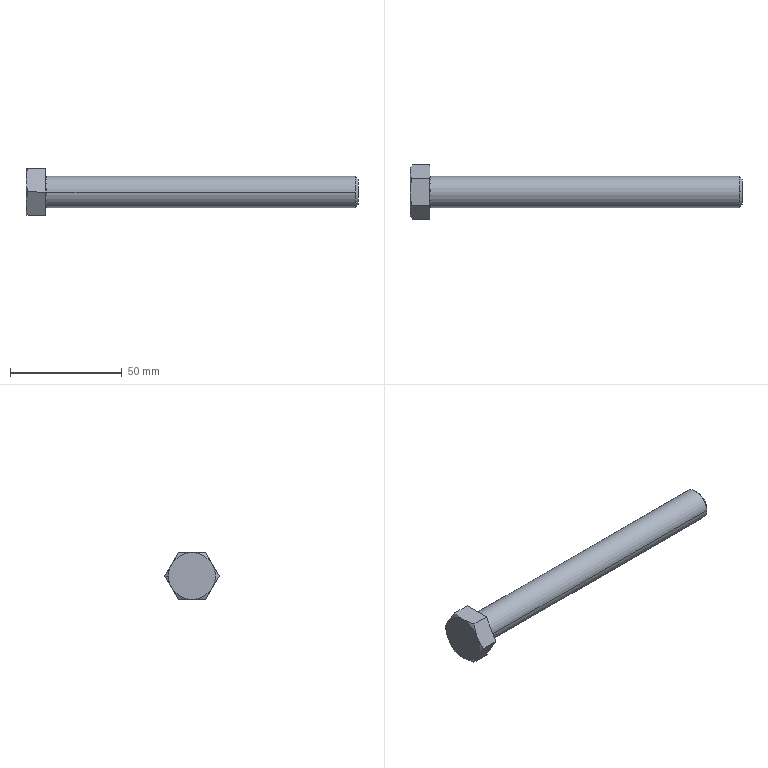Part | SolidWorks | features BaseBody 1 | 1 solid | 22 faces | box 148.8 x 24.249 x 21 mm | volume 24876 mm3 | cone 9 | plane 9 | spline 2 | cylinder 2 | commonest cylinder face diameters 14 x2
STEP:
#1=CARTESIAN_POINT('',(0.,0.,7.6));
#2=VERTEX_POINT('',#1);
#3=CARTESIAN_POINT('',(0.,0.,-7.6));
#4=VERTEX_POINT('',#3);
#5=CARTESIAN_POINT('',(0.,0.,7.6));
#6=CARTESIAN_POINT('',(0.,0.2323,7.6));
#7=CARTESIAN_POINT('',(0.,0.5793,7.584));
#8=CARTESIAN_POINT('',(0.,0.9819,7.538));
#9=CARTESIAN_POINT('',(0.,1.183,7.508));
#10=CARTESIAN_POINT('',(0.,1.268,7.493));
#11=CARTESIAN_POINT('',(0.,1.326,7.484));
#12=CARTESIAN_POINT('',(0.,1.353,7.479));
#13=CARTESIAN_POINT('',(0.,1.625,7.428));
#14=CARTESIAN_POINT('',(0.,1.984,7.344));
#15=CARTESIAN_POINT('',(0.,2.393,7.215));
#16=CARTESIAN_POINT('',(0.,2.596,7.143));
#17=CARTESIAN_POINT('',(0.,2.683,7.111));
#18=CARTESIAN_POINT('',(0.,2.74,7.089));
#19=CARTESIAN_POINT('',(0.,2.768,7.078));
#20=CARTESIAN_POINT('',(0.,3.036,6.972));
#21=CARTESIAN_POINT('',(0.,3.385,6.813));
#22=CARTESIAN_POINT('',(0.,3.777,6.597));
#23=CARTESIAN_POINT('',(0.,3.942,6.498));
#24=CARTESIAN_POINT('',(0.,4.051,6.431));
#25=CARTESIAN_POINT('',(0.,4.104,6.397));
#26=CARTESIAN_POINT('',(0.,4.598,6.074));
#27=CARTESIAN_POINT('',(0.,5.003,5.745));
#28=CARTESIAN_POINT('',(0.,5.559,5.189));
#29=CARTESIAN_POINT('',(0.,5.822,4.898));
#30=CARTESIAN_POINT('',(0.,6.101,4.536));
#31=CARTESIAN_POINT('',(0.,6.214,4.376));
#32=CARTESIAN_POINT('',(0.,6.289,4.268));
#33=CARTESIAN_POINT('',(0.,6.326,4.212));
#34=CARTESIAN_POINT('',(0.,6.502,3.944));
#35=CARTESIAN_POINT('',(0.,6.695,3.613));
#36=CARTESIAN_POINT('',(0.,6.891,3.21));
#37=CARTESIAN_POINT('',(0.,6.981,3.005));
#38=CARTESIAN_POINT('',(0.,7.018,2.917));
#39=CARTESIAN_POINT('',(0.,7.043,2.857));
#40=CARTESIAN_POINT('',(0.,7.055,2.826));
#41=CARTESIAN_POINT('',(0.,7.157,2.569));
#42=CARTESIAN_POINT('',(0.,7.276,2.22));
#43=CARTESIAN_POINT('',(0.,7.385,1.804));
#44=CARTESIAN_POINT('',(0.,7.431,1.594));
#45=CARTESIAN_POINT('',(0.,7.45,1.504));
#46=CARTESIAN_POINT('',(0.,7.462,1.443));
#47=CARTESIAN_POINT('',(0.,7.468,1.411));
#48=CARTESIAN_POINT('',(0.,7.558,0.9257));
#49=CARTESIAN_POINT('',(0.,7.6,0.4647));
#50=CARTESIAN_POINT('',(0.,7.6,-0.2323));
#51=CARTESIAN_POINT('',(0.,7.589,-0.464));
#52=CARTESIAN_POINT('',(0.,7.558,-0.8097));
#53=CARTESIAN_POINT('',(0.,7.538,-0.9822));
#54=CARTESIAN_POINT('',(0.,7.508,-1.183));
#55=CARTESIAN_POINT('',(0.,7.493,-1.269));
#56=CARTESIAN_POINT('',(0.,7.484,-1.326));
#57=CARTESIAN_POINT('',(0.,7.479,-1.353));
#58=CARTESIAN_POINT('',(0.,7.428,-1.625));
#59=CARTESIAN_POINT('',(0.,7.344,-1.984));
#60=CARTESIAN_POINT('',(0.,7.215,-2.393));
#61=CARTESIAN_POINT('',(0.,7.143,-2.596));
#62=CARTESIAN_POINT('',(0.,7.111,-2.683));
#63=CARTESIAN_POINT('',(0.,7.089,-2.74));
#64=CARTESIAN_POINT('',(0.,7.078,-2.768));
#65=CARTESIAN_POINT('',(0.,6.972,-3.036));
#66=CARTESIAN_POINT('',(0.,6.813,-3.385));
#67=CARTESIAN_POINT('',(0.,6.597,-3.777));
#68=CARTESIAN_POINT('',(0.,6.498,-3.942));
#69=CARTESIAN_POINT('',(0.,6.431,-4.051));
#70=CARTESIAN_POINT('',(0.,6.397,-4.104));
#71=CARTESIAN_POINT('',(0.,6.074,-4.598));
#72=CARTESIAN_POINT('',(0.,5.745,-5.003));
#73=CARTESIAN_POINT('',(0.,5.189,-5.559));
#74=CARTESIAN_POINT('',(0.,4.898,-5.822));
#75=CARTESIAN_POINT('',(0.,4.536,-6.101));
#76=CARTESIAN_POINT('',(0.,4.376,-6.214));
#77=CARTESIAN_POINT('',(0.,4.268,-6.289));
#78=CARTESIAN_POINT('',(0.,4.212,-6.326));
#79=CARTESIAN_POINT('',(0.,3.944,-6.502));
#80=CARTESIAN_POINT('',(0.,3.613,-6.695));
#81=CARTESIAN_POINT('',(0.,3.21,-6.891));
#82=CARTESIAN_POINT('',(0.,3.005,-6.981));
#83=CARTESIAN_POINT('',(0.,2.917,-7.018));
#84=CARTESIAN_POINT('',(0.,2.857,-7.043));
#85=CARTESIAN_POINT('',(0.,2.826,-7.055));
#86=CARTESIAN_POINT('',(0.,2.569,-7.157));
#87=CARTESIAN_POINT('',(0.,2.22,-7.276));
#88=CARTESIAN_POINT('',(0.,1.804,-7.385));
#89=CARTESIAN_POINT('',(0.,1.594,-7.431));
#90=CARTESIAN_POINT('',(0.,1.504,-7.45));
#91=CARTESIAN_POINT('',(0.,1.443,-7.462));
#92=CARTESIAN_POINT('',(0.,1.411,-7.468));
#93=CARTESIAN_POINT('',(0.,0.9262,-7.558));
#94=CARTESIAN_POINT('',(0.,0.4645,-7.6));
#95=CARTESIAN_POINT('',(0.,0.,-7.6));
#96=B_SPLINE_CURVE_WITH_KNOTS('',3,(#5,#6,#7,#8,#9,#10,#11,#12,#13,#14,#15,#16,#17,#18,#19,#20,#21,#22,#23,#24,#25,#26,#27,#28,#29,#30,#31,#32,#33,#34,#35,#36,#37,#38,#39,#40,#41,#42,#43,#44,#45,#46,#47,#48,#49,#50,#51,#52,#53,#54,#55,#56,#57,#58,#59,#60,#61,#62,#63,#64,#65,#66,#67,#68,#69,#70,#71,#72,#73,#74,#75,#76,#77,#78,#79,#80,#81,#82,#83,#84,#85,#86,#87,#88,#89,#90,#91,#92,#93,#94,#95),.UNSPECIFIED.,.F.,.F.,(4,1,1,1,2,2,1,1,1,2,2,1,1,2,2,2,1,1,2,2,1,1,1,2,2,1,1,1,2,2,2,2,1,1,2,2,1,1,1,2,2,1,1,2,2,2,1,1,2,2,1,1,1,2,2,1,1,1,2,2,4),(0.75,0.7656,0.7734,0.7773,0.7793,0.7812,0.7969,0.8047,0.8086,0.8105,0.8125,0.8281,0.8359,0.8398,0.8438,0.875,0.8906,0.8984,0.9023,0.9063,0.9219,0.9297,0.9336,0.9355,0.9375,0.9531,0.9609,0.9648,0.9668,0.9688,1.,1.016,1.023,1.027,1.029,1.031,1.047,1.055,1.059,1.061,1.063,1.078,1.086,1.09,1.094,1.125,1.141,1.148,1.152,1.156,1.172,1.18,1.184,1.186,1.188,1.203,1.211,1.215,1.217,1.219,1.25),.UNSPECIFIED.);
#97=EDGE_CURVE('',#2,#4,#96,.T.);
#98=ORIENTED_EDGE('',*,*,#97,.F.);
#99=CARTESIAN_POINT('',(0.6,0.,7.));
#100=VERTEX_POINT('',#99);
#101=CARTESIAN_POINT('',(0.6,0.,7.6));
#102=DIRECTION('',(0.,-1.,0.));
#103=DIRECTION('',(0.,0.,1.));
#104=AXIS2_PLACEMENT_3D('',#101,#102,#103);
#105=CIRCLE('',#104,0.6);
#106=EDGE_CURVE('',#2,#100,#105,.T.);
#107=ORIENTED_EDGE('',*,*,#106,.T.);
#108=CARTESIAN_POINT('',(0.6,7.,0.));
#109=VERTEX_POINT('',#108);
#110=CARTESIAN_POINT('',(0.6,0.,0.));
#111=DIRECTION('',(1.,0.,0.));
#112=DIRECTION('',(0.,1.,0.));
#113=AXIS2_PLACEMENT_3D('',#110,#111,#112);
#114=CIRCLE('',#113,7.);
#115=EDGE_CURVE('',#109,#100,#114,.T.);
#116=ORIENTED_EDGE('',*,*,#115,.F.);
#117=CARTESIAN_POINT('',(0.6,0.,-7.));
#118=VERTEX_POINT('',#117);
#119=CARTESIAN_POINT('',(0.6,0.,0.));
#120=DIRECTION('',(1.,0.,0.));
#121=DIRECTION('',(0.,1.,0.));
#122=AXIS2_PLACEMENT_3D('',#119,#120,#121);
#123=CIRCLE('',#122,7.);
#124=EDGE_CURVE('',#118,#109,#123,.T.);
#125=ORIENTED_EDGE('',*,*,#124,.F.);
#126=CARTESIAN_POINT('',(0.6,0.,-7.6));
#127=DIRECTION('',(0.,1.,0.));
#128=DIRECTION('',(0.,0.,-1.));
#129=AXIS2_PLACEMENT_3D('',#126,#127,#128);
#130=CIRCLE('',#129,0.6);
#131=EDGE_CURVE('',#4,#118,#130,.T.);
#132=ORIENTED_EDGE('',*,*,#131,.F.);
#133=EDGE_LOOP('',(#98,#107,#116,#125,#132));
#134=FACE_OUTER_BOUND('',#133,.T.);
#135=CARTESIAN_POINT('',(0.,0.,-7.6));
#136=CARTESIAN_POINT('',(0.,15.2,-7.6));
#137=CARTESIAN_POINT('',(0.,15.2,7.6));
#138=CARTESIAN_POINT('',(0.,0.,7.6));
#139=CARTESIAN_POINT('',(0.,0.,-7.249));
#140=CARTESIAN_POINT('',(0.,14.497,-7.249));
#141=CARTESIAN_POINT('',(0.,14.497,7.249));
#142=CARTESIAN_POINT('',(0.,0.,7.249));
#143=CARTESIAN_POINT('',(0.2485,0.,-7.));
#144=CARTESIAN_POINT('',(0.2485,14.,-7.));
#145=CARTESIAN_POINT('',(0.2485,14.,7.));
#146=CARTESIAN_POINT('',(0.2485,0.,7.));
#147=CARTESIAN_POINT('',(0.6,0.,-7.));
#148=CARTESIAN_POINT('',(0.6,14.,-7.));
#149=CARTESIAN_POINT('',(0.6,14.,7.));
#150=CARTESIAN_POINT('',(0.6,0.,7.));
#151=(BOUNDED_SURFACE()B_SPLINE_SURFACE(3,3,((#135,#136,#137,#138),(#139,#140,#141,#142),(#143,#144,#145,#146),(#147,#148,#149,#150)),.UNSPECIFIED.,.F.,.F.,.F.)B_SPLINE_SURFACE_WITH_KNOTS((4,4),(4,4),(0.,1.),(0.,1.),.UNSPECIFIED.)GEOMETRIC_REPRESENTATION_ITEM()RATIONAL_B_SPLINE_SURFACE(((1.,0.3333,0.3333,1.),(0.8047,0.2682,0.2682,0.8047),(0.8047,0.2682,0.2682,0.8047),(1.,0.3333,0.3333,1.)))REPRESENTATION_ITEM('')SURFACE());
#152=ADVANCED_FACE('',(#134),#151,.F.);
#153=ORIENTED_EDGE('',*,*,#115,.T.);
#154=CARTESIAN_POINT('',(0.6,-7.,0.));
#155=VERTEX_POINT('',#154);
#156=CARTESIAN_POINT('',(0.6,0.,0.));
#157=DIRECTION('',(1.,0.,0.));
#158=DIRECTION('',(0.,1.,0.));
#159=AXIS2_PLACEMENT_3D('',#156,#157,#158);
#160=CIRCLE('',#159,7.);
#161=EDGE_CURVE('',#100,#155,#160,.T.);
#162=ORIENTED_EDGE('',*,*,#161,.T.);
#163=CARTESIAN_POINT('',(138.773,-7.,0.));
#164=VERTEX_POINT('',#163);
#165=CARTESIAN_POINT('',(70.,-7.,0.));
#166=DIRECTION('',(1.,0.,0.));
#167=VECTOR('',#166,1000.);
#168=LINE('',#165,#167);
#169=EDGE_CURVE('',#155,#164,#168,.T.);
#170=ORIENTED_EDGE('',*,*,#169,.T.);
#171=CARTESIAN_POINT('',(138.773,0.,7.));
#172=VERTEX_POINT('',#171);
#173=CARTESIAN_POINT('',(138.773,0.,0.));
#174=DIRECTION('',(-1.,0.,0.));
#175=DIRECTION('',(0.,1.,0.));
#176=AXIS2_PLACEMENT_3D('',#173,#174,#175);
#177=CIRCLE('',#176,7.);
#178=EDGE_CURVE('',#164,#172,#177,.T.);
#179=ORIENTED_EDGE('',*,*,#178,.T.);
#180=CARTESIAN_POINT('',(138.773,7.,0.));
#181=VERTEX_POINT('',#180);
#182=CARTESIAN_POINT('',(138.773,0.,0.));
#183=DIRECTION('',(-1.,0.,0.));
#184=DIRECTION('',(0.,1.,0.));
#185=AXIS2_PLACEMENT_3D('',#182,#183,#184);
#186=CIRCLE('',#185,7.);
#187=EDGE_CURVE('',#172,#181,#186,.T.);
#188=ORIENTED_EDGE('',*,*,#187,.T.);
#189=CARTESIAN_POINT('',(70.,7.,0.));
#190=DIRECTION('',(1.,0.,0.));
#191=VECTOR('',#190,1000.);
#192=LINE('',#189,#191);
#193=EDGE_CURVE('',#109,#181,#192,.T.);
#194=ORIENTED_EDGE('',*,*,#193,.F.);
#195=EDGE_LOOP('',(#153,#162,#170,#179,#188,#194));
#196=FACE_OUTER_BOUND('',#195,.T.);
#197=CARTESIAN_POINT('',(70.,0.,0.));
#198=DIRECTION('',(1.,0.,0.));
#199=DIRECTION('',(0.,1.,0.));
#200=AXIS2_PLACEMENT_3D('',#197,#198,#199);
#201=CYLINDRICAL_SURFACE('',#200,7.);
#202=ADVANCED_FACE('',(#196),#201,.T.);
#203=CARTESIAN_POINT('',(140.,0.,5.773));
#204=VERTEX_POINT('',#203);
#205=CARTESIAN_POINT('',(140.,0.,-5.773));
#206=VERTEX_POINT('',#205);
#207=CARTESIAN_POINT('',(140.,0.,0.));
#208=DIRECTION('',(-1.,0.,0.));
#209=DIRECTION('',(0.,0.,1.));
#210=AXIS2_PLACEMENT_3D('',#207,#208,#209);
#211=CIRCLE('',#210,5.773);
#212=EDGE_CURVE('',#204,#206,#211,.T.);
#213=ORIENTED_EDGE('',*,*,#212,.T.);
#214=CARTESIAN_POINT('',(138.773,0.,-7.));
#215=VERTEX_POINT('',#214);
#216=CARTESIAN_POINT('',(138.773,0.,-7.));
#217=DIRECTION('',(-0.7071,0.,-0.7071));
#218=VECTOR('',#217,1000.);
#219=LINE('',#216,#218);
#220=EDGE_CURVE('',#206,#215,#219,.T.);
#221=ORIENTED_EDGE('',*,*,#220,.T.);
#222=CARTESIAN_POINT('',(138.773,0.,0.));
#223=DIRECTION('',(-1.,0.,0.));
#224=DIRECTION('',(0.,1.,0.));
#225=AXIS2_PLACEMENT_3D('',#222,#223,#224);
#226=CIRCLE('',#225,7.);
#227=EDGE_CURVE('',#181,#215,#226,.T.);
#228=ORIENTED_EDGE('',*,*,#227,.F.);
#229=ORIENTED_EDGE('',*,*,#187,.F.);
#230=CARTESIAN_POINT('',(138.773,0.,7.));
#231=DIRECTION('',(-0.7071,0.,0.7071));
#232=VECTOR('',#231,1000.);
#233=LINE('',#230,#232);
#234=EDGE_CURVE('',#204,#172,#233,.T.);
#235=ORIENTED_EDGE('',*,*,#234,.F.);
#236=EDGE_LOOP('',(#213,#221,#228,#229,#235));
#237=FACE_OUTER_BOUND('',#236,.T.);
#238=CARTESIAN_POINT('',(138.773,0.,0.));
#239=DIRECTION('',(-1.,0.,0.));
#240=DIRECTION('',(0.,0.,1.));
#241=AXIS2_PLACEMENT_3D('',#238,#239,#240);
#242=CONICAL_SURFACE('',#241,7.,0.7854);
#243=ADVANCED_FACE('',(#237),#242,.T.);
#244=CARTESIAN_POINT('',(-8.8,9.093,-5.25));
#245=VERTEX_POINT('',#244);
#246=CARTESIAN_POINT('',(-8.8,10.5,0.));
#247=VERTEX_POINT('',#246);
#248=CARTESIAN_POINT('',(-8.8,0.,0.));
#249=DIRECTION('',(1.,0.,0.));
#250=DIRECTION('',(0.,1.,0.));
#251=AXIS2_PLACEMENT_3D('',#248,#249,#250);
#252=CIRCLE('',#251,10.5);
#253=EDGE_CURVE('',#245,#247,#252,.T.);
#254=ORIENTED_EDGE('',*,*,#253,.T.);
#255=CARTESIAN_POINT('',(-7.862,12.124,0.));
#256=VERTEX_POINT('',#255);
#257=CARTESIAN_POINT('',(-7.857,12.134,0.));
#258=DIRECTION('',(0.5,0.866,0.));
#259=VECTOR('',#258,1000.);
#260=LINE('',#257,#259);
#261=EDGE_CURVE('',#247,#256,#260,.T.);
#262=ORIENTED_EDGE('',*,*,#261,.T.);
#263=CARTESIAN_POINT('',(-8.8,9.093,-5.25));
#264=CARTESIAN_POINT('',(-8.8,9.611,-4.354));
#265=CARTESIAN_POINT('',(-8.71,10.121,-3.47));
#266=CARTESIAN_POINT('',(-8.384,11.13,-1.722));
#267=CARTESIAN_POINT('',(-8.148,11.629,-0.8576));
#268=CARTESIAN_POINT('',(-7.862,12.124,0.));
#269=B_SPLINE_CURVE_WITH_KNOTS('',3,(#263,#264,#265,#266,#267,#268),.UNSPECIFIED.,.F.,.F.,(4,2,4),(0.,0.003067,0.006134),.UNSPECIFIED.);
#270=EDGE_CURVE('',#245,#256,#269,.T.);
#271=ORIENTED_EDGE('',*,*,#270,.F.);
#272=EDGE_LOOP('',(#254,#262,#271));
#273=FACE_OUTER_BOUND('',#272,.T.);
#274=CARTESIAN_POINT('',(-7.857,0.,0.));
#275=DIRECTION('',(1.,0.,0.));
#276=DIRECTION('',(0.,1.,0.));
#277=AXIS2_PLACEMENT_3D('',#274,#275,#276);
#278=CONICAL_SURFACE('',#277,12.134,1.047);
#279=ADVANCED_FACE('',(#273),#278,.T.);
#280=ORIENTED_EDGE('',*,*,#169,.F.);
#281=CARTESIAN_POINT('',(0.6,0.,0.));
#282=DIRECTION('',(1.,0.,0.));
#283=DIRECTION('',(0.,1.,0.));
#284=AXIS2_PLACEMENT_3D('',#281,#282,#283);
#285=CIRCLE('',#284,7.);
#286=EDGE_CURVE('',#155,#118,#285,.T.);
#287=ORIENTED_EDGE('',*,*,#286,.T.);
#288=ORIENTED_EDGE('',*,*,#124,.T.);
#289=ORIENTED_EDGE('',*,*,#193,.T.);
#290=ORIENTED_EDGE('',*,*,#227,.T.);
#291=CARTESIAN_POINT('',(138.773,0.,0.));
#292=DIRECTION('',(-1.,0.,0.));
#293=DIRECTION('',(0.,1.,0.));
#294=AXIS2_PLACEMENT_3D('',#291,#292,#293);
#295=CIRCLE('',#294,7.);
#296=EDGE_CURVE('',#215,#164,#295,.T.);
#297=ORIENTED_EDGE('',*,*,#296,.T.);
#298=EDGE_LOOP('',(#280,#287,#288,#289,#290,#297));
#299=FACE_OUTER_BOUND('',#298,.T.);
#300=CARTESIAN_POINT('',(70.,0.,0.));
#301=DIRECTION('',(1.,0.,0.));
#302=DIRECTION('',(0.,1.,0.));
#303=AXIS2_PLACEMENT_3D('',#300,#301,#302);
#304=CYLINDRICAL_SURFACE('',#303,7.);
#305=ADVANCED_FACE('',(#299),#304,.T.);
#306=ORIENTED_EDGE('',*,*,#106,.F.);
#307=CARTESIAN_POINT('',(0.,0.,-7.6));
#308=CARTESIAN_POINT('',(0.,-0.2323,-7.6));
#309=CARTESIAN_POINT('',(0.,-0.5793,-7.584));
#310=CARTESIAN_POINT('',(0.,-0.9819,-7.538));
#311=CARTESIAN_POINT('',(0.,-1.183,-7.508));
#312=CARTESIAN_POINT('',(0.,-1.268,-7.493));
#313=CARTESIAN_POINT('',(0.,-1.326,-7.484));
#314=CARTESIAN_POINT('',(0.,-1.353,-7.479));
#315=CARTESIAN_POINT('',(0.,-1.625,-7.428));
#316=CARTESIAN_POINT('',(0.,-1.984,-7.344));
#317=CARTESIAN_POINT('',(0.,-2.393,-7.215));
#318=CARTESIAN_POINT('',(0.,-2.596,-7.143));
#319=CARTESIAN_POINT('',(0.,-2.683,-7.111));
#320=CARTESIAN_POINT('',(0.,-2.74,-7.089));
#321=CARTESIAN_POINT('',(0.,-2.768,-7.078));
#322=CARTESIAN_POINT('',(0.,-3.036,-6.972));
#323=CARTESIAN_POINT('',(0.,-3.385,-6.813));
#324=CARTESIAN_POINT('',(0.,-3.777,-6.597));
#325=CARTESIAN_POINT('',(0.,-3.942,-6.498));
#326=CARTESIAN_POINT('',(0.,-4.051,-6.431));
#327=CARTESIAN_POINT('',(0.,-4.104,-6.397));
#328=CARTESIAN_POINT('',(0.,-4.598,-6.074));
#329=CARTESIAN_POINT('',(0.,-5.003,-5.745));
#330=CARTESIAN_POINT('',(0.,-5.559,-5.189));
#331=CARTESIAN_POINT('',(0.,-5.822,-4.898));
#332=CARTESIAN_POINT('',(0.,-6.101,-4.536));
#333=CARTESIAN_POINT('',(0.,-6.214,-4.376));
#334=CARTESIAN_POINT('',(0.,-6.289,-4.268));
#335=CARTESIAN_POINT('',(0.,-6.326,-4.212));
#336=CARTESIAN_POINT('',(0.,-6.502,-3.944));
#337=CARTESIAN_POINT('',(0.,-6.695,-3.613));
#338=CARTESIAN_POINT('',(0.,-6.891,-3.21));
#339=CARTESIAN_POINT('',(0.,-6.981,-3.005));
#340=CARTESIAN_POINT('',(0.,-7.018,-2.917));
#341=CARTESIAN_POINT('',(0.,-7.043,-2.857));
#342=CARTESIAN_POINT('',(0.,-7.055,-2.826));
#343=CARTESIAN_POINT('',(0.,-7.157,-2.569));
#344=CARTESIAN_POINT('',(0.,-7.276,-2.22));
#345=CARTESIAN_POINT('',(0.,-7.385,-1.804));
#346=CARTESIAN_POINT('',(0.,-7.431,-1.594));
#347=CARTESIAN_POINT('',(0.,-7.45,-1.504));
#348=CARTESIAN_POINT('',(0.,-7.462,-1.443));
#349=CARTESIAN_POINT('',(0.,-7.468,-1.411));
#350=CARTESIAN_POINT('',(0.,-7.558,-0.9262));
#351=CARTESIAN_POINT('',(0.,-7.6,-0.4645));
#352=CARTESIAN_POINT('',(0.,-7.6,0.2323));
#353=CARTESIAN_POINT('',(0.,-7.584,0.5793));
#354=CARTESIAN_POINT('',(0.,-7.538,0.9819));
#355=CARTESIAN_POINT('',(0.,-7.508,1.183));
#356=CARTESIAN_POINT('',(0.,-7.493,1.268));
#357=CARTESIAN_POINT('',(0.,-7.484,1.326));
#358=CARTESIAN_POINT('',(0.,-7.479,1.353));
#359=CARTESIAN_POINT('',(0.,-7.428,1.625));
#360=CARTESIAN_POINT('',(0.,-7.344,1.984));
#361=CARTESIAN_POINT('',(0.,-7.215,2.393));
#362=CARTESIAN_POINT('',(0.,-7.143,2.596));
#363=CARTESIAN_POINT('',(0.,-7.111,2.683));
#364=CARTESIAN_POINT('',(0.,-7.089,2.74));
#365=CARTESIAN_POINT('',(0.,-7.078,2.768));
#366=CARTESIAN_POINT('',(0.,-6.972,3.036));
#367=CARTESIAN_POINT('',(0.,-6.813,3.385));
#368=CARTESIAN_POINT('',(0.,-6.597,3.777));
#369=CARTESIAN_POINT('',(0.,-6.498,3.942));
#370=CARTESIAN_POINT('',(0.,-6.431,4.051));
#371=CARTESIAN_POINT('',(0.,-6.397,4.104));
#372=CARTESIAN_POINT('',(0.,-6.074,4.598));
#373=CARTESIAN_POINT('',(0.,-5.745,5.003));
#374=CARTESIAN_POINT('',(0.,-5.189,5.559));
#375=CARTESIAN_POINT('',(0.,-4.898,5.822));
#376=CARTESIAN_POINT('',(0.,-4.536,6.101));
#377=CARTESIAN_POINT('',(0.,-4.376,6.214));
#378=CARTESIAN_POINT('',(0.,-4.268,6.289));
#379=CARTESIAN_POINT('',(0.,-4.212,6.326));
#380=CARTESIAN_POINT('',(0.,-3.944,6.502));
#381=CARTESIAN_POINT('',(0.,-3.613,6.695));
#382=CARTESIAN_POINT('',(0.,-3.21,6.891));
#383=CARTESIAN_POINT('',(0.,-3.005,6.981));
#384=CARTESIAN_POINT('',(0.,-2.917,7.018));
#385=CARTESIAN_POINT('',(0.,-2.857,7.043));
#386=CARTESIAN_POINT('',(0.,-2.826,7.055));
#387=CARTESIAN_POINT('',(0.,-2.569,7.157));
#388=CARTESIAN_POINT('',(0.,-2.22,7.276));
#389=CARTESIAN_POINT('',(0.,-1.804,7.385));
#390=CARTESIAN_POINT('',(0.,-1.594,7.431));
#391=CARTESIAN_POINT('',(0.,-1.504,7.45));
#392=CARTESIAN_POINT('',(0.,-1.443,7.462));
#393=CARTESIAN_POINT('',(0.,-1.411,7.468));
#394=CARTESIAN_POINT('',(0.,-0.9262,7.558));
#395=CARTESIAN_POINT('',(0.,-0.4645,7.6));
#396=CARTESIAN_POINT('',(0.,0.,7.6));
#397=B_SPLINE_CURVE_WITH_KNOTS('',3,(#307,#308,#309,#310,#311,#312,#313,#314,#315,#316,#317,#318,#319,#320,#321,#322,#323,#324,#325,#326,#327,#328,#329,#330,#331,#332,#333,#334,#335,#336,#337,#338,#339,#340,#341,#342,#343,#344,#345,#346,#347,#348,#349,#350,#351,#352,#353,#354,#355,#356,#357,#358,#359,#360,#361,#362,#363,#364,#365,#366,#367,#368,#369,#370,#371,#372,#373,#374,#375,#376,#377,#378,#379,#380,#381,#382,#383,#384,#385,#386,#387,#388,#389,#390,#391,#392,#393,#394,#395,#396),.UNSPECIFIED.,.F.,.F.,(4,1,1,1,2,2,1,1,1,2,2,1,1,2,2,2,1,1,2,2,1,1,1,2,2,1,1,1,2,2,2,1,1,1,2,2,1,1,1,2,2,1,1,2,2,2,1,1,2,2,1,1,1,2,2,1,1,1,2,2,4),(0.25,0.2656,0.2734,0.2773,0.2793,0.2812,0.2969,0.3047,0.3086,0.3105,0.3125,0.3281,0.3359,0.3398,0.3437,0.375,0.3906,0.3984,0.4023,0.4062,0.4219,0.4297,0.4336,0.4355,0.4375,0.4531,0.4609,0.4648,0.4668,0.4687,0.5,0.5156,0.5234,0.5273,0.5293,0.5312,0.5469,0.5547,0.5586,0.5605,0.5625,0.5781,0.5859,0.5898,0.5938,0.625,0.6406,0.6484,0.6523,0.6562,0.6719,0.6797,0.6836,0.6855,0.6875,0.7031,0.7109,0.7148,0.7168,0.7188,0.75),.UNSPECIFIED.);
#398=EDGE_CURVE('',#4,#2,#397,.T.);
#399=ORIENTED_EDGE('',*,*,#398,.F.);
#400=ORIENTED_EDGE('',*,*,#131,.T.);
#401=ORIENTED_EDGE('',*,*,#286,.F.);
#402=ORIENTED_EDGE('',*,*,#161,.F.);
#403=EDGE_LOOP('',(#306,#399,#400,#401,#402));
#404=FACE_OUTER_BOUND('',#403,.T.);
#405=CARTESIAN_POINT('',(0.,0.,7.6));
#406=CARTESIAN_POINT('',(0.,-15.2,7.6));
#407=CARTESIAN_POINT('',(0.,-15.2,-7.6));
#408=CARTESIAN_POINT('',(0.,0.,-7.6));
#409=CARTESIAN_POINT('',(0.,0.,7.249));
#410=CARTESIAN_POINT('',(0.,-14.497,7.249));
#411=CARTESIAN_POINT('',(0.,-14.497,-7.249));
#412=CARTESIAN_POINT('',(0.,0.,-7.249));
#413=CARTESIAN_POINT('',(0.2485,0.,7.));
#414=CARTESIAN_POINT('',(0.2485,-14.,7.));
#415=CARTESIAN_POINT('',(0.2485,-14.,-7.));
#416=CARTESIAN_POINT('',(0.2485,0.,-7.));
#417=CARTESIAN_POINT('',(0.6,0.,7.));
#418=CARTESIAN_POINT('',(0.6,-14.,7.));
#419=CARTESIAN_POINT('',(0.6,-14.,-7.));
#420=CARTESIAN_POINT('',(0.6,0.,-7.));
#421=(BOUNDED_SURFACE()B_SPLINE_SURFACE(3,3,((#405,#406,#407,#408),(#409,#410,#411,#412),(#413,#414,#415,#416),(#417,#418,#419,#420)),.UNSPECIFIED.,.F.,.F.,.F.)B_SPLINE_SURFACE_WITH_KNOTS((4,4),(4,4),(0.,1.),(0.,1.),.UNSPECIFIED.)GEOMETRIC_REPRESENTATION_ITEM()RATIONAL_B_SPLINE_SURFACE(((1.,0.3333,0.3333,1.),(0.8047,0.2682,0.2682,0.8047),(0.8047,0.2682,0.2682,0.8047),(1.,0.3333,0.3333,1.)))REPRESENTATION_ITEM('')SURFACE());
#422=ADVANCED_FACE('',(#404),#421,.F.);
#423=ORIENTED_EDGE('',*,*,#220,.F.);
#424=CARTESIAN_POINT('',(140.,0.,0.));
#425=DIRECTION('',(-1.,0.,0.));
#426=DIRECTION('',(0.,0.,1.));
#427=AXIS2_PLACEMENT_3D('',#424,#425,#426);
#428=CIRCLE('',#427,5.773);
#429=EDGE_CURVE('',#206,#204,#428,.T.);
#430=ORIENTED_EDGE('',*,*,#429,.T.);
#431=ORIENTED_EDGE('',*,*,#234,.T.);
#432=ORIENTED_EDGE('',*,*,#178,.F.);
#433=ORIENTED_EDGE('',*,*,#296,.F.);
#434=EDGE_LOOP('',(#423,#430,#431,#432,#433));
#435=FACE_OUTER_BOUND('',#434,.T.);
#436=CARTESIAN_POINT('',(138.773,0.,0.));
#437=DIRECTION('',(-1.,0.,0.));
#438=DIRECTION('',(0.,0.,1.));
#439=AXIS2_PLACEMENT_3D('',#436,#437,#438);
#440=CONICAL_SURFACE('',#439,7.,0.7854);
#441=ADVANCED_FACE('',(#435),#440,.T.);
#442=ORIENTED_EDGE('',*,*,#398,.T.);
#443=ORIENTED_EDGE('',*,*,#97,.T.);
#444=EDGE_LOOP('',(#442,#443));
#445=FACE_BOUND('',#444,.T.);
#446=CARTESIAN_POINT('',(0.,-6.062,-10.5));
#447=VERTEX_POINT('',#446);
#448=CARTESIAN_POINT('',(0.,6.062,-10.5));
#449=VERTEX_POINT('',#448);
#450=CARTESIAN_POINT('',(0.,0.,-10.5));
#451=DIRECTION('',(0.,1.,0.));
#452=VECTOR('',#451,1000.);
#453=LINE('',#450,#452);
#454=EDGE_CURVE('',#447,#449,#453,.T.);
#455=ORIENTED_EDGE('',*,*,#454,.T.);
#456=CARTESIAN_POINT('',(0.,12.124,0.));
#457=VERTEX_POINT('',#456);
#458=CARTESIAN_POINT('',(0.,6.062,-10.5));
#459=DIRECTION('',(0.,0.5,0.866));
#460=VECTOR('',#459,1000.);
#461=LINE('',#458,#460);
#462=EDGE_CURVE('',#449,#457,#461,.T.);
#463=ORIENTED_EDGE('',*,*,#462,.T.);
#464=CARTESIAN_POINT('',(0.,6.062,10.5));
#465=VERTEX_POINT('',#464);
#466=CARTESIAN_POINT('',(0.,12.124,0.));
#467=DIRECTION('',(0.,-0.5,0.866));
#468=VECTOR('',#467,1000.);
#469=LINE('',#466,#468);
#470=EDGE_CURVE('',#457,#465,#469,.T.);
#471=ORIENTED_EDGE('',*,*,#470,.T.);
#472=CARTESIAN_POINT('',(0.,-6.062,10.5));
#473=VERTEX_POINT('',#472);
#474=CARTESIAN_POINT('',(0.,0.,10.5));
#475=DIRECTION('',(0.,-1.,0.));
#476=VECTOR('',#475,1000.);
#477=LINE('',#474,#476);
#478=EDGE_CURVE('',#465,#473,#477,.T.);
#479=ORIENTED_EDGE('',*,*,#478,.T.);
#480=CARTESIAN_POINT('',(0.,-12.124,0.));
#481=VERTEX_POINT('',#480);
#482=CARTESIAN_POINT('',(0.,-6.062,10.5));
#483=DIRECTION('',(0.,-0.5,-0.866));
#484=VECTOR('',#483,1000.);
#485=LINE('',#482,#484);
#486=EDGE_CURVE('',#473,#481,#485,.T.);
#487=ORIENTED_EDGE('',*,*,#486,.T.);
#488=CARTESIAN_POINT('',(0.,-12.124,0.));
#489=DIRECTION('',(0.,0.5,-0.866));
#490=VECTOR('',#489,1000.);
#491=LINE('',#488,#490);
#492=EDGE_CURVE('',#481,#447,#491,.T.);
#493=ORIENTED_EDGE('',*,*,#492,.T.);
#494=EDGE_LOOP('',(#455,#463,#471,#479,#487,#493));
#495=FACE_OUTER_BOUND('',#494,.T.);
#496=CARTESIAN_POINT('',(0.,0.,0.));
#497=DIRECTION('',(1.,0.,0.));
#498=DIRECTION('',(0.,1.,0.));
#499=AXIS2_PLACEMENT_3D('',#496,#497,#498);
#500=PLANE('',#499);
#501=ADVANCED_FACE('',(#445,#495),#500,.T.);
#502=ORIENTED_EDGE('',*,*,#212,.F.);
#503=ORIENTED_EDGE('',*,*,#429,.F.);
#504=EDGE_LOOP('',(#502,#503));
#505=FACE_OUTER_BOUND('',#504,.T.);
#506=CARTESIAN_POINT('',(140.,3.5,0.));
#507=DIRECTION('',(1.,0.,0.));
#508=DIRECTION('',(0.,1.,0.));
#509=AXIS2_PLACEMENT_3D('',#506,#507,#508);
#510=PLANE('',#509);
#511=ADVANCED_FACE('',(#505),#510,.T.);
#512=CARTESIAN_POINT('',(-7.862,6.062,-10.5));
#513=VERTEX_POINT('',#512);
#514=CARTESIAN_POINT('',(0.,6.062,-10.5));
#515=DIRECTION('',(-1.,0.,0.));
#516=VECTOR('',#515,1000.);
#517=LINE('',#514,#516);
#518=EDGE_CURVE('',#449,#513,#517,.T.);
#519=ORIENTED_EDGE('',*,*,#518,.T.);
#520=CARTESIAN_POINT('',(-7.862,6.062,-10.5));
#521=CARTESIAN_POINT('',(-8.148,6.557,-9.642));
#522=CARTESIAN_POINT('',(-8.384,7.056,-8.778));
#523=CARTESIAN_POINT('',(-8.71,8.066,-7.03));
#524=CARTESIAN_POINT('',(-8.8,8.576,-6.146));
#525=CARTESIAN_POINT('',(-8.8,9.093,-5.25));
#526=B_SPLINE_CURVE_WITH_KNOTS('',3,(#520,#521,#522,#523,#524,#525),.UNSPECIFIED.,.F.,.F.,(4,2,4),(0.,0.003067,0.006134),.UNSPECIFIED.);
#527=EDGE_CURVE('',#513,#245,#526,.T.);
#528=ORIENTED_EDGE('',*,*,#527,.T.);
#529=ORIENTED_EDGE('',*,*,#270,.T.);
#530=CARTESIAN_POINT('',(0.,12.124,0.));
#531=DIRECTION('',(1.,0.,0.));
#532=VECTOR('',#531,1000.);
#533=LINE('',#530,#532);
#534=EDGE_CURVE('',#256,#457,#533,.T.);
#535=ORIENTED_EDGE('',*,*,#534,.T.);
#536=ORIENTED_EDGE('',*,*,#462,.F.);
#537=EDGE_LOOP('',(#519,#528,#529,#535,#536));
#538=FACE_OUTER_BOUND('',#537,.T.);
#539=CARTESIAN_POINT('',(0.,6.062,-10.5));
#540=DIRECTION('',(0.,0.866,-0.5));
#541=DIRECTION('',(0.,0.5,0.866));
#542=AXIS2_PLACEMENT_3D('',#539,#540,#541);
#543=PLANE('',#542);
#544=ADVANCED_FACE('',(#538),#543,.T.);
#545=ORIENTED_EDGE('',*,*,#454,.F.);
#546=CARTESIAN_POINT('',(-7.862,-6.062,-10.5));
#547=VERTEX_POINT('',#546);
#548=CARTESIAN_POINT('',(0.,-6.062,-10.5));
#549=DIRECTION('',(-1.,0.,0.));
#550=VECTOR('',#549,1000.);
#551=LINE('',#548,#550);
#552=EDGE_CURVE('',#447,#547,#551,.T.);
#553=ORIENTED_EDGE('',*,*,#552,.T.);
#554=CARTESIAN_POINT('',(-8.8,0.,-10.5));
#555=VERTEX_POINT('',#554);
#556=CARTESIAN_POINT('',(-7.862,-6.062,-10.5));
#557=CARTESIAN_POINT('',(-8.148,-5.072,-10.5));
#558=CARTESIAN_POINT('',(-8.384,-4.074,-10.5));
#559=CARTESIAN_POINT('',(-8.71,-2.055,-10.5));
#560=CARTESIAN_POINT('',(-8.8,-1.035,-10.5));
#561=CARTESIAN_POINT('',(-8.8,0.,-10.5));
#562=B_SPLINE_CURVE_WITH_KNOTS('',3,(#556,#557,#558,#559,#560,#561),.UNSPECIFIED.,.F.,.F.,(4,2,4),(0.,0.003067,0.006134),.UNSPECIFIED.);
#563=EDGE_CURVE('',#547,#555,#562,.T.);
#564=ORIENTED_EDGE('',*,*,#563,.T.);
#565=CARTESIAN_POINT('',(-8.8,0.,-10.5));
#566=CARTESIAN_POINT('',(-8.8,1.035,-10.5));
#567=CARTESIAN_POINT('',(-8.71,2.055,-10.5));
#568=CARTESIAN_POINT('',(-8.384,4.074,-10.5));
#569=CARTESIAN_POINT('',(-8.148,5.072,-10.5));
#570=CARTESIAN_POINT('',(-7.862,6.062,-10.5));
#571=B_SPLINE_CURVE_WITH_KNOTS('',3,(#565,#566,#567,#568,#569,#570),.UNSPECIFIED.,.F.,.F.,(4,2,4),(0.,0.003067,0.006134),.UNSPECIFIED.);
#572=EDGE_CURVE('',#555,#513,#571,.T.);
#573=ORIENTED_EDGE('',*,*,#572,.T.);
#574=ORIENTED_EDGE('',*,*,#518,.F.);
#575=EDGE_LOOP('',(#545,#553,#564,#573,#574));
#576=FACE_OUTER_BOUND('',#575,.T.);
#577=CARTESIAN_POINT('',(0.,-6.062,-10.5));
#578=DIRECTION('',(0.,0.,-1.));
#579=DIRECTION('',(0.,1.,0.));
#580=AXIS2_PLACEMENT_3D('',#577,#578,#579);
#581=PLANE('',#580);
#582=ADVANCED_FACE('',(#576),#581,.T.);
#583=ORIENTED_EDGE('',*,*,#492,.F.);
#584=CARTESIAN_POINT('',(-7.862,-12.124,0.));
#585=VERTEX_POINT('',#584);
#586=CARTESIAN_POINT('',(0.,-12.124,0.));
#587=DIRECTION('',(-1.,0.,0.));
#588=VECTOR('',#587,1000.);
#589=LINE('',#586,#588);
#590=EDGE_CURVE('',#481,#585,#589,.T.);
#591=ORIENTED_EDGE('',*,*,#590,.T.);
#592=CARTESIAN_POINT('',(-8.8,-9.093,-5.25));
#593=VERTEX_POINT('',#592);
#594=CARTESIAN_POINT('',(-7.862,-12.124,0.));
#595=CARTESIAN_POINT('',(-8.148,-11.629,-0.8576));
#596=CARTESIAN_POINT('',(-8.384,-11.13,-1.722));
#597=CARTESIAN_POINT('',(-8.71,-10.121,-3.47));
#598=CARTESIAN_POINT('',(-8.8,-9.611,-4.354));
#599=CARTESIAN_POINT('',(-8.8,-9.093,-5.25));
#600=B_SPLINE_CURVE_WITH_KNOTS('',3,(#594,#595,#596,#597,#598,#599),.UNSPECIFIED.,.F.,.F.,(4,2,4),(0.,0.003067,0.006134),.UNSPECIFIED.);
#601=EDGE_CURVE('',#585,#593,#600,.T.);
#602=ORIENTED_EDGE('',*,*,#601,.T.);
#603=CARTESIAN_POINT('',(-8.8,-9.093,-5.25));
#604=CARTESIAN_POINT('',(-8.8,-8.576,-6.146));
#605=CARTESIAN_POINT('',(-8.71,-8.066,-7.03));
#606=CARTESIAN_POINT('',(-8.384,-7.056,-8.778));
#607=CARTESIAN_POINT('',(-8.148,-6.557,-9.642));
#608=CARTESIAN_POINT('',(-7.862,-6.062,-10.5));
#609=B_SPLINE_CURVE_WITH_KNOTS('',3,(#603,#604,#605,#606,#607,#608),.UNSPECIFIED.,.F.,.F.,(4,2,4),(0.,0.003067,0.006134),.UNSPECIFIED.);
#610=EDGE_CURVE('',#593,#547,#609,.T.);
#611=ORIENTED_EDGE('',*,*,#610,.T.);
#612=ORIENTED_EDGE('',*,*,#552,.F.);
#613=EDGE_LOOP('',(#583,#591,#602,#611,#612));
#614=FACE_OUTER_BOUND('',#613,.T.);
#615=CARTESIAN_POINT('',(0.,-12.124,0.));
#616=DIRECTION('',(0.,-0.866,-0.5));
#617=DIRECTION('',(0.,0.5,-0.866));
#618=AXIS2_PLACEMENT_3D('',#615,#616,#617);
#619=PLANE('',#618);
#620=ADVANCED_FACE('',(#614),#619,.T.);
#621=ORIENTED_EDGE('',*,*,#486,.F.);
#622=CARTESIAN_POINT('',(-7.862,-6.062,10.5));
#623=VERTEX_POINT('',#622);
#624=CARTESIAN_POINT('',(0.,-6.062,10.5));
#625=DIRECTION('',(-1.,0.,0.));
#626=VECTOR('',#625,1000.);
#627=LINE('',#624,#626);
#628=EDGE_CURVE('',#473,#623,#627,.T.);
#629=ORIENTED_EDGE('',*,*,#628,.T.);
#630=CARTESIAN_POINT('',(-8.8,-9.093,5.25));
#631=VERTEX_POINT('',#630);
#632=CARTESIAN_POINT('',(-7.862,-6.062,10.5));
#633=CARTESIAN_POINT('',(-8.148,-6.557,9.642));
#634=CARTESIAN_POINT('',(-8.384,-7.056,8.778));
#635=CARTESIAN_POINT('',(-8.71,-8.066,7.03));
#636=CARTESIAN_POINT('',(-8.8,-8.576,6.146));
#637=CARTESIAN_POINT('',(-8.8,-9.093,5.25));
#638=B_SPLINE_CURVE_WITH_KNOTS('',3,(#632,#633,#634,#635,#636,#637),.UNSPECIFIED.,.F.,.F.,(4,2,4),(0.,0.003067,0.006134),.UNSPECIFIED.);
#639=EDGE_CURVE('',#623,#631,#638,.T.);
#640=ORIENTED_EDGE('',*,*,#639,.T.);
#641=CARTESIAN_POINT('',(-8.8,-9.093,5.25));
#642=CARTESIAN_POINT('',(-8.8,-9.611,4.354));
#643=CARTESIAN_POINT('',(-8.71,-10.121,3.47));
#644=CARTESIAN_POINT('',(-8.384,-11.13,1.722));
#645=CARTESIAN_POINT('',(-8.148,-11.629,0.8576));
#646=CARTESIAN_POINT('',(-7.862,-12.124,0.));
#647=B_SPLINE_CURVE_WITH_KNOTS('',3,(#641,#642,#643,#644,#645,#646),.UNSPECIFIED.,.F.,.F.,(4,2,4),(0.,0.003067,0.006134),.UNSPECIFIED.);
#648=EDGE_CURVE('',#631,#585,#647,.T.);
#649=ORIENTED_EDGE('',*,*,#648,.T.);
#650=ORIENTED_EDGE('',*,*,#590,.F.);
#651=EDGE_LOOP('',(#621,#629,#640,#649,#650));
#652=FACE_OUTER_BOUND('',#651,.T.);
#653=CARTESIAN_POINT('',(0.,-6.062,10.5));
#654=DIRECTION('',(0.,-0.866,0.5));
#655=DIRECTION('',(0.,-0.5,-0.866));
#656=AXIS2_PLACEMENT_3D('',#653,#654,#655);
#657=PLANE('',#656);
#658=ADVANCED_FACE('',(#652),#657,.T.);
#659=CARTESIAN_POINT('',(-7.862,6.062,10.5));
#660=VERTEX_POINT('',#659);
#661=CARTESIAN_POINT('',(0.,6.062,10.5));
#662=DIRECTION('',(-1.,0.,0.));
#663=VECTOR('',#662,1000.);
#664=LINE('',#661,#663);
#665=EDGE_CURVE('',#465,#660,#664,.T.);
#666=ORIENTED_EDGE('',*,*,#665,.T.);
#667=CARTESIAN_POINT('',(-8.8,0.,10.5));
#668=VERTEX_POINT('',#667);
#669=CARTESIAN_POINT('',(-7.862,6.062,10.5));
#670=CARTESIAN_POINT('',(-8.148,5.072,10.5));
#671=CARTESIAN_POINT('',(-8.384,4.074,10.5));
#672=CARTESIAN_POINT('',(-8.71,2.055,10.5));
#673=CARTESIAN_POINT('',(-8.8,1.035,10.5));
#674=CARTESIAN_POINT('',(-8.8,0.,10.5));
#675=B_SPLINE_CURVE_WITH_KNOTS('',3,(#669,#670,#671,#672,#673,#674),.UNSPECIFIED.,.F.,.F.,(4,2,4),(0.,0.003067,0.006134),.UNSPECIFIED.);
#676=EDGE_CURVE('',#660,#668,#675,.T.);
#677=ORIENTED_EDGE('',*,*,#676,.T.);
#678=CARTESIAN_POINT('',(-8.8,0.,10.5));
#679=CARTESIAN_POINT('',(-8.8,-1.035,10.5));
#680=CARTESIAN_POINT('',(-8.71,-2.055,10.5));
#681=CARTESIAN_POINT('',(-8.384,-4.074,10.5));
#682=CARTESIAN_POINT('',(-8.148,-5.072,10.5));
#683=CARTESIAN_POINT('',(-7.862,-6.062,10.5));
#684=B_SPLINE_CURVE_WITH_KNOTS('',3,(#678,#679,#680,#681,#682,#683),.UNSPECIFIED.,.F.,.F.,(4,2,4),(0.,0.003067,0.006134),.UNSPECIFIED.);
#685=EDGE_CURVE('',#668,#623,#684,.T.);
#686=ORIENTED_EDGE('',*,*,#685,.T.);
#687=ORIENTED_EDGE('',*,*,#628,.F.);
#688=ORIENTED_EDGE('',*,*,#478,.F.);
#689=EDGE_LOOP('',(#666,#677,#686,#687,#688));
#690=FACE_OUTER_BOUND('',#689,.T.);
#691=CARTESIAN_POINT('',(0.,6.062,10.5));
#692=DIRECTION('',(0.,0.,1.));
#693=DIRECTION('',(0.,-1.,0.));
#694=AXIS2_PLACEMENT_3D('',#691,#692,#693);
#695=PLANE('',#694);
#696=ADVANCED_FACE('',(#690),#695,.T.);
#697=ORIENTED_EDGE('',*,*,#534,.F.);
#698=CARTESIAN_POINT('',(-8.8,9.093,5.25));
#699=VERTEX_POINT('',#698);
#700=CARTESIAN_POINT('',(-7.862,12.124,0.));
#701=CARTESIAN_POINT('',(-8.148,11.629,0.8576));
#702=CARTESIAN_POINT('',(-8.384,11.13,1.722));
#703=CARTESIAN_POINT('',(-8.71,10.121,3.47));
#704=CARTESIAN_POINT('',(-8.8,9.611,4.354));
#705=CARTESIAN_POINT('',(-8.8,9.093,5.25));
#706=B_SPLINE_CURVE_WITH_KNOTS('',3,(#700,#701,#702,#703,#704,#705),.UNSPECIFIED.,.F.,.F.,(4,2,4),(0.,0.003067,0.006134),.UNSPECIFIED.);
#707=EDGE_CURVE('',#256,#699,#706,.T.);
#708=ORIENTED_EDGE('',*,*,#707,.T.);
#709=CARTESIAN_POINT('',(-8.8,9.093,5.25));
#710=CARTESIAN_POINT('',(-8.8,8.576,6.146));
#711=CARTESIAN_POINT('',(-8.71,8.066,7.03));
#712=CARTESIAN_POINT('',(-8.384,7.056,8.778));
#713=CARTESIAN_POINT('',(-8.148,6.557,9.642));
#714=CARTESIAN_POINT('',(-7.862,6.062,10.5));
#715=B_SPLINE_CURVE_WITH_KNOTS('',3,(#709,#710,#711,#712,#713,#714),.UNSPECIFIED.,.F.,.F.,(4,2,4),(0.,0.003067,0.006134),.UNSPECIFIED.);
#716=EDGE_CURVE('',#699,#660,#715,.T.);
#717=ORIENTED_EDGE('',*,*,#716,.T.);
#718=ORIENTED_EDGE('',*,*,#665,.F.);
#719=ORIENTED_EDGE('',*,*,#470,.F.);
#720=EDGE_LOOP('',(#697,#708,#717,#718,#719));
#721=FACE_OUTER_BOUND('',#720,.T.);
#722=CARTESIAN_POINT('',(0.,12.124,0.));
#723=DIRECTION('',(0.,0.866,0.5));
#724=DIRECTION('',(0.,-0.5,0.866));
#725=AXIS2_PLACEMENT_3D('',#722,#723,#724);
#726=PLANE('',#725);
#727=ADVANCED_FACE('',(#721),#726,.T.);
#728=CARTESIAN_POINT('',(-8.8,0.,0.));
#729=DIRECTION('',(1.,0.,0.));
#730=DIRECTION('',(0.,1.,0.));
#731=AXIS2_PLACEMENT_3D('',#728,#729,#730);
#732=CIRCLE('',#731,10.5);
#733=EDGE_CURVE('',#555,#245,#732,.T.);
#734=ORIENTED_EDGE('',*,*,#733,.T.);
#735=ORIENTED_EDGE('',*,*,#527,.F.);
#736=ORIENTED_EDGE('',*,*,#572,.F.);
#737=EDGE_LOOP('',(#734,#735,#736));
#738=FACE_OUTER_BOUND('',#737,.T.);
#739=CARTESIAN_POINT('',(-7.857,0.,0.));
#740=DIRECTION('',(1.,0.,0.));
#741=DIRECTION('',(0.,1.,0.));
#742=AXIS2_PLACEMENT_3D('',#739,#740,#741);
#743=CONICAL_SURFACE('',#742,12.134,1.047);
#744=ADVANCED_FACE('',(#738),#743,.T.);
#745=ORIENTED_EDGE('',*,*,#261,.F.);
#746=CARTESIAN_POINT('',(-8.8,0.,0.));
#747=DIRECTION('',(1.,0.,0.));
#748=DIRECTION('',(0.,1.,0.));
#749=AXIS2_PLACEMENT_3D('',#746,#747,#748);
#750=CIRCLE('',#749,10.5);
#751=EDGE_CURVE('',#247,#699,#750,.T.);
#752=ORIENTED_EDGE('',*,*,#751,.T.);
#753=ORIENTED_EDGE('',*,*,#707,.F.);
#754=EDGE_LOOP('',(#745,#752,#753));
#755=FACE_OUTER_BOUND('',#754,.T.);
#756=CARTESIAN_POINT('',(-7.857,0.,0.));
#757=DIRECTION('',(1.,0.,0.));
#758=DIRECTION('',(0.,1.,0.));
#759=AXIS2_PLACEMENT_3D('',#756,#757,#758);
#760=CONICAL_SURFACE('',#759,12.134,1.047);
#761=ADVANCED_FACE('',(#755),#760,.T.);
#762=CARTESIAN_POINT('',(-8.8,0.,0.));
#763=DIRECTION('',(1.,0.,0.));
#764=DIRECTION('',(0.,1.,0.));
#765=AXIS2_PLACEMENT_3D('',#762,#763,#764);
#766=CIRCLE('',#765,10.5);
#767=EDGE_CURVE('',#593,#555,#766,.T.);
#768=ORIENTED_EDGE('',*,*,#767,.T.);
#769=ORIENTED_EDGE('',*,*,#563,.F.);
#770=ORIENTED_EDGE('',*,*,#610,.F.);
#771=EDGE_LOOP('',(#768,#769,#770));
#772=FACE_OUTER_BOUND('',#771,.T.);
#773=CARTESIAN_POINT('',(-7.857,0.,0.));
#774=DIRECTION('',(1.,0.,0.));
#775=DIRECTION('',(0.,1.,0.));
#776=AXIS2_PLACEMENT_3D('',#773,#774,#775);
#777=CONICAL_SURFACE('',#776,12.134,1.047);
#778=ADVANCED_FACE('',(#772),#777,.T.);
#779=CARTESIAN_POINT('',(-8.8,0.,0.));
#780=DIRECTION('',(1.,0.,0.));
#781=DIRECTION('',(0.,1.,0.));
#782=AXIS2_PLACEMENT_3D('',#779,#780,#781);
#783=CIRCLE('',#782,10.5);
#784=EDGE_CURVE('',#631,#593,#783,.T.);
#785=ORIENTED_EDGE('',*,*,#784,.T.);
#786=ORIENTED_EDGE('',*,*,#601,.F.);
#787=ORIENTED_EDGE('',*,*,#648,.F.);
#788=EDGE_LOOP('',(#785,#786,#787));
#789=FACE_OUTER_BOUND('',#788,.T.);
#790=CARTESIAN_POINT('',(-7.857,0.,0.));
#791=DIRECTION('',(1.,0.,0.));
#792=DIRECTION('',(0.,1.,0.));
#793=AXIS2_PLACEMENT_3D('',#790,#791,#792);
#794=CONICAL_SURFACE('',#793,12.134,1.047);
#795=ADVANCED_FACE('',(#789),#794,.T.);
#796=ORIENTED_EDGE('',*,*,#685,.F.);
#797=CARTESIAN_POINT('',(-8.8,0.,0.));
#798=DIRECTION('',(1.,0.,0.));
#799=DIRECTION('',(0.,1.,0.));
#800=AXIS2_PLACEMENT_3D('',#797,#798,#799);
#801=CIRCLE('',#800,10.5);
#802=EDGE_CURVE('',#668,#631,#801,.T.);
#803=ORIENTED_EDGE('',*,*,#802,.T.);
#804=ORIENTED_EDGE('',*,*,#639,.F.);
#805=EDGE_LOOP('',(#796,#803,#804));
#806=FACE_OUTER_BOUND('',#805,.T.);
#807=CARTESIAN_POINT('',(-7.857,0.,0.));
#808=DIRECTION('',(1.,0.,0.));
#809=DIRECTION('',(0.,1.,0.));
#810=AXIS2_PLACEMENT_3D('',#807,#808,#809);
#811=CONICAL_SURFACE('',#810,12.134,1.047);
#812=ADVANCED_FACE('',(#806),#811,.T.);
#813=ORIENTED_EDGE('',*,*,#716,.F.);
#814=CARTESIAN_POINT('',(-8.8,0.,0.));
#815=DIRECTION('',(1.,0.,0.));
#816=DIRECTION('',(0.,1.,0.));
#817=AXIS2_PLACEMENT_3D('',#814,#815,#816);
#818=CIRCLE('',#817,10.5);
#819=EDGE_CURVE('',#699,#668,#818,.T.);
#820=ORIENTED_EDGE('',*,*,#819,.T.);
#821=ORIENTED_EDGE('',*,*,#676,.F.);
#822=EDGE_LOOP('',(#813,#820,#821));
#823=FACE_OUTER_BOUND('',#822,.T.);
#824=CARTESIAN_POINT('',(-7.857,0.,0.));
#825=DIRECTION('',(1.,0.,0.));
#826=DIRECTION('',(0.,1.,0.));
#827=AXIS2_PLACEMENT_3D('',#824,#825,#826);
#828=CONICAL_SURFACE('',#827,12.134,1.047);
#829=ADVANCED_FACE('',(#823),#828,.T.);
#830=ORIENTED_EDGE('',*,*,#767,.F.);
#831=ORIENTED_EDGE('',*,*,#784,.F.);
#832=ORIENTED_EDGE('',*,*,#802,.F.);
#833=ORIENTED_EDGE('',*,*,#819,.F.);
#834=ORIENTED_EDGE('',*,*,#751,.F.);
#835=ORIENTED_EDGE('',*,*,#253,.F.);
#836=ORIENTED_EDGE('',*,*,#733,.F.);
#837=EDGE_LOOP('',(#830,#831,#832,#833,#834,#835,#836));
#838=FACE_OUTER_BOUND('',#837,.T.);
#839=CARTESIAN_POINT('',(-8.8,0.,0.));
#840=DIRECTION('',(1.,0.,0.));
#841=DIRECTION('',(0.,1.,0.));
#842=AXIS2_PLACEMENT_3D('',#839,#840,#841);
#843=PLANE('',#842);
#844=ADVANCED_FACE('',(#838),#843,.F.);
#845=CLOSED_SHELL('',(#152,#202,#243,#279,#305,#422,#441,#501,#511,#544,#582,#620,#658,#696,#727,#744,#761,#778,#795,#812,#829,#844));
#846=MANIFOLD_SOLID_BREP('',#845);
#847=CARTESIAN_POINT('',(0.,0.,0.));
#848=DIRECTION('',(0.,0.,1.));
#849=DIRECTION('',(1.,0.,0.));
#850=AXIS2_PLACEMENT_3D('',#847,#848,#849);
#851=(LENGTH_UNIT()NAMED_UNIT(*)SI_UNIT(.MILLI.,.METRE.));
#852=UNCERTAINTY_MEASURE_WITH_UNIT(LENGTH_MEASURE(0.00001),#851,'','');
#853=(NAMED_UNIT(*)PLANE_ANGLE_UNIT()SI_UNIT($,.RADIAN.));
#854=(NAMED_UNIT(*)SI_UNIT($,.STERADIAN.)SOLID_ANGLE_UNIT());
#855=(GEOMETRIC_REPRESENTATION_CONTEXT(3)GLOBAL_UNCERTAINTY_ASSIGNED_CONTEXT((#852))GLOBAL_UNIT_ASSIGNED_CONTEXT((#851,#853,#854))REPRESENTATION_CONTEXT('',''));
#856=ADVANCED_BREP_SHAPE_REPRESENTATION('',(#846,#850),#855);